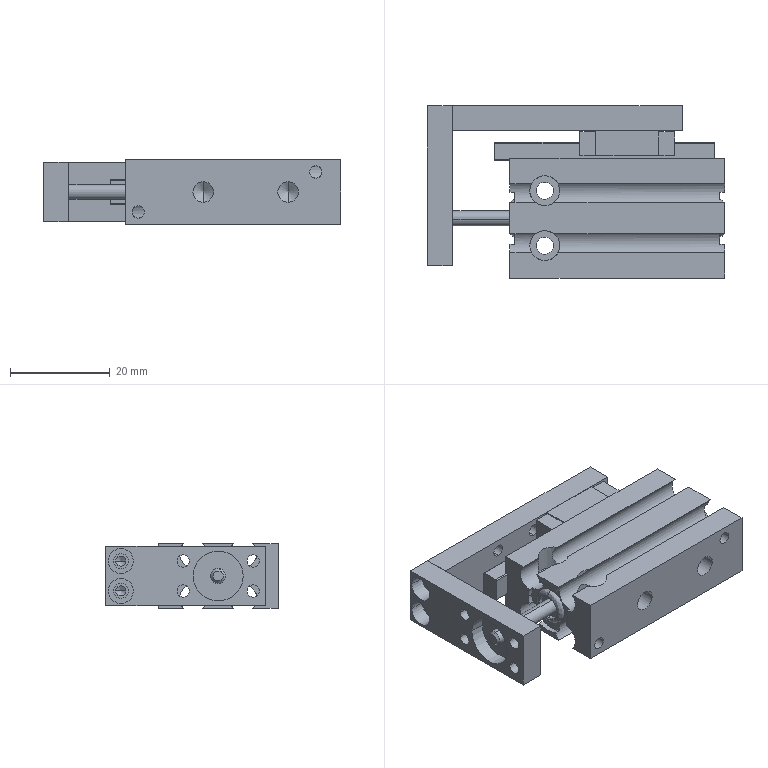Part | SolidWorks | 6 solids | 210 faces | box 59.5 x 34.5 x 13 mm | volume 14643 mm3 | cylinder 106 | plane 80 | cone 20 | spline 4 | commonest cylinder face diameters 2.459 x20 3 x14 5 x12 6 x12 11 x10 5.5 x8